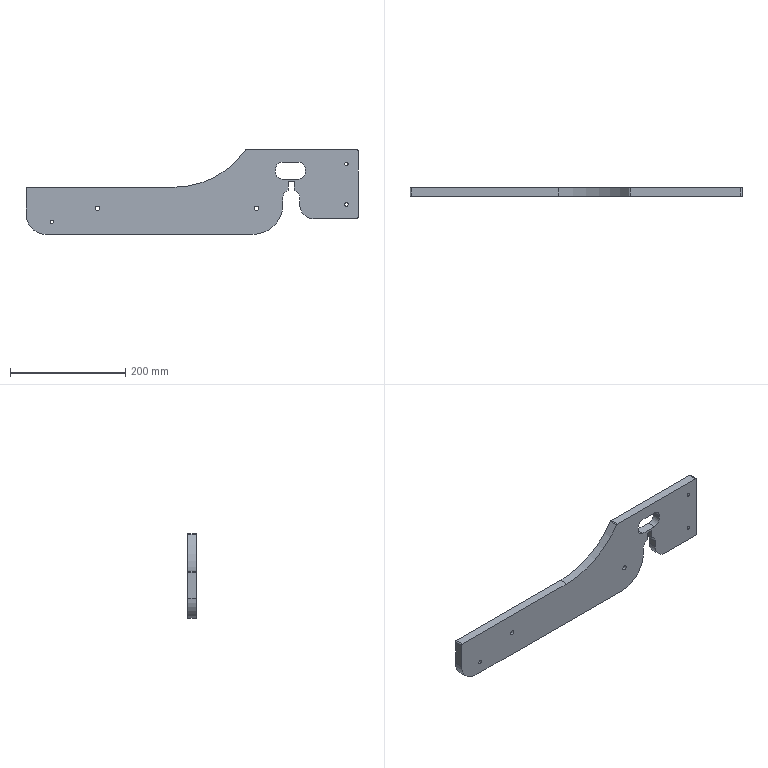Part | STEP file | Left | 1 solid | 80 faces | box 575 x 15 x 147 mm | volume 816987 mm3 | plane 43 | cylinder 19 | other 18 | commonest cylinder face diameters 4 x4 24 x4 6 x3 8 x2 29 x2 50 x1